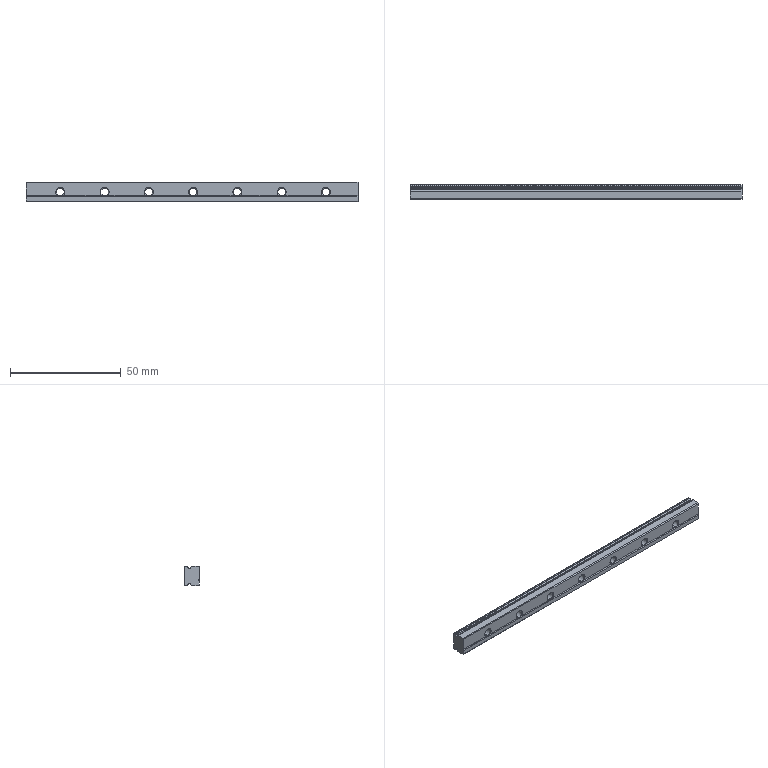Part | STEP file | _Rail-MGN9R01501HM-7.5 | 1 solid | 99 faces | box 150 x 6.5 x 9 mm | volume 7402 mm3 | cylinder 45 | cone 28 | plane 26 | commonest cylinder face diameters 3.5 x14 6 x14 0.3 x12 2 x4 1 x1